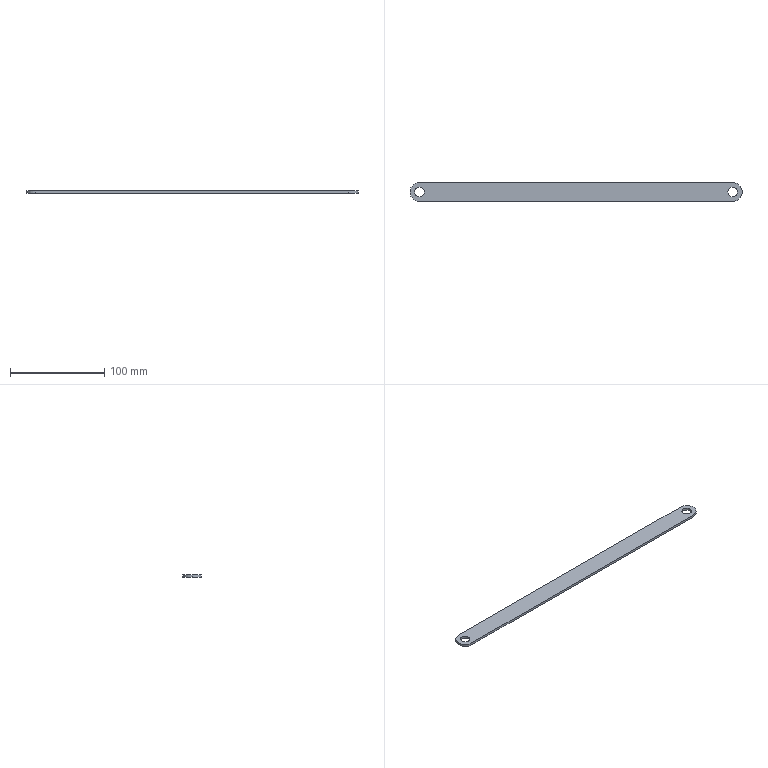Part | SolidWorks | features Extrusion 1 | 1 solid | 11 faces | box 351.77 x 20 x 2.5 mm | volume 16981 mm3 | cylinder 7 | plane 4 | commonest cylinder face diameters 10 x4 20 x3
STEP:
#1=CARTESIAN_POINT('',(160.885,0.,2.5));
#2=VERTEX_POINT('',#1);
#3=CARTESIAN_POINT('',(170.885,0.,2.5));
#4=VERTEX_POINT('',#3);
#5=CARTESIAN_POINT('',(165.885,0.,2.5));
#6=DIRECTION('',(0.,0.,1.));
#7=DIRECTION('',(1.,0.,0.));
#8=AXIS2_PLACEMENT_3D('',#5,#6,#7);
#9=CIRCLE('',#8,5.);
#10=EDGE_CURVE('',#2,#4,#9,.T.);
#11=ORIENTED_EDGE('',*,*,#10,.T.);
#12=CARTESIAN_POINT('',(170.885,0.,0.));
#13=VERTEX_POINT('',#12);
#14=CARTESIAN_POINT('',(170.885,0.,2.5));
#15=DIRECTION('',(0.,0.,-1.));
#16=VECTOR('',#15,1000.);
#17=LINE('',#14,#16);
#18=EDGE_CURVE('',#4,#13,#17,.T.);
#19=ORIENTED_EDGE('',*,*,#18,.T.);
#20=CARTESIAN_POINT('',(160.885,0.,0.));
#21=VERTEX_POINT('',#20);
#22=CARTESIAN_POINT('',(165.885,0.,0.));
#23=DIRECTION('',(0.,0.,1.));
#24=DIRECTION('',(1.,0.,0.));
#25=AXIS2_PLACEMENT_3D('',#22,#23,#24);
#26=CIRCLE('',#25,5.);
#27=EDGE_CURVE('',#21,#13,#26,.T.);
#28=ORIENTED_EDGE('',*,*,#27,.F.);
#29=CARTESIAN_POINT('',(160.885,0.,2.5));
#30=DIRECTION('',(0.,0.,-1.));
#31=VECTOR('',#30,1000.);
#32=LINE('',#29,#31);
#33=EDGE_CURVE('',#2,#21,#32,.T.);
#34=ORIENTED_EDGE('',*,*,#33,.F.);
#35=EDGE_LOOP('',(#11,#19,#28,#34));
#36=FACE_OUTER_BOUND('',#35,.T.);
#37=CARTESIAN_POINT('',(165.885,0.,2.5));
#38=DIRECTION('',(0.,0.,-1.));
#39=DIRECTION('',(-1.,0.,0.));
#40=AXIS2_PLACEMENT_3D('',#37,#38,#39);
#41=CYLINDRICAL_SURFACE('',#40,5.);
#42=ADVANCED_FACE('',(#36),#41,.F.);
#43=CARTESIAN_POINT('',(-170.885,0.,2.5));
#44=VERTEX_POINT('',#43);
#45=CARTESIAN_POINT('',(-160.885,0.,2.5));
#46=VERTEX_POINT('',#45);
#47=CARTESIAN_POINT('',(-165.885,0.,2.5));
#48=DIRECTION('',(0.,0.,1.));
#49=DIRECTION('',(1.,0.,0.));
#50=AXIS2_PLACEMENT_3D('',#47,#48,#49);
#51=CIRCLE('',#50,5.);
#52=EDGE_CURVE('',#44,#46,#51,.T.);
#53=ORIENTED_EDGE('',*,*,#52,.T.);
#54=CARTESIAN_POINT('',(-160.885,0.,0.));
#55=VERTEX_POINT('',#54);
#56=CARTESIAN_POINT('',(-160.885,0.,2.5));
#57=DIRECTION('',(0.,0.,-1.));
#58=VECTOR('',#57,1000.);
#59=LINE('',#56,#58);
#60=EDGE_CURVE('',#46,#55,#59,.T.);
#61=ORIENTED_EDGE('',*,*,#60,.T.);
#62=CARTESIAN_POINT('',(-170.885,0.,0.));
#63=VERTEX_POINT('',#62);
#64=CARTESIAN_POINT('',(-165.885,0.,0.));
#65=DIRECTION('',(0.,0.,1.));
#66=DIRECTION('',(1.,0.,0.));
#67=AXIS2_PLACEMENT_3D('',#64,#65,#66);
#68=CIRCLE('',#67,5.);
#69=EDGE_CURVE('',#63,#55,#68,.T.);
#70=ORIENTED_EDGE('',*,*,#69,.F.);
#71=CARTESIAN_POINT('',(-170.885,0.,2.5));
#72=DIRECTION('',(0.,0.,-1.));
#73=VECTOR('',#72,1000.);
#74=LINE('',#71,#73);
#75=EDGE_CURVE('',#44,#63,#74,.T.);
#76=ORIENTED_EDGE('',*,*,#75,.F.);
#77=EDGE_LOOP('',(#53,#61,#70,#76));
#78=FACE_OUTER_BOUND('',#77,.T.);
#79=CARTESIAN_POINT('',(-165.885,0.,2.5));
#80=DIRECTION('',(0.,0.,-1.));
#81=DIRECTION('',(-1.,0.,0.));
#82=AXIS2_PLACEMENT_3D('',#79,#80,#81);
#83=CYLINDRICAL_SURFACE('',#82,5.);
#84=ADVANCED_FACE('',(#78),#83,.F.);
#85=CARTESIAN_POINT('',(-175.885,0.,2.5));
#86=VERTEX_POINT('',#85);
#87=CARTESIAN_POINT('',(-165.885,-10.,2.5));
#88=VERTEX_POINT('',#87);
#89=CARTESIAN_POINT('',(-165.885,0.,2.5));
#90=DIRECTION('',(0.,0.,1.));
#91=DIRECTION('',(1.,0.,0.));
#92=AXIS2_PLACEMENT_3D('',#89,#90,#91);
#93=CIRCLE('',#92,10.);
#94=EDGE_CURVE('',#86,#88,#93,.T.);
#95=ORIENTED_EDGE('',*,*,#94,.F.);
#96=CARTESIAN_POINT('',(-175.885,0.,0.));
#97=VERTEX_POINT('',#96);
#98=CARTESIAN_POINT('',(-175.885,0.,2.5));
#99=DIRECTION('',(0.,0.,-1.));
#100=VECTOR('',#99,1000.);
#101=LINE('',#98,#100);
#102=EDGE_CURVE('',#86,#97,#101,.T.);
#103=ORIENTED_EDGE('',*,*,#102,.T.);
#104=CARTESIAN_POINT('',(-165.885,-10.,0.));
#105=VERTEX_POINT('',#104);
#106=CARTESIAN_POINT('',(-165.885,0.,0.));
#107=DIRECTION('',(0.,0.,1.));
#108=DIRECTION('',(1.,0.,0.));
#109=AXIS2_PLACEMENT_3D('',#106,#107,#108);
#110=CIRCLE('',#109,10.);
#111=EDGE_CURVE('',#97,#105,#110,.T.);
#112=ORIENTED_EDGE('',*,*,#111,.T.);
#113=CARTESIAN_POINT('',(-165.885,-10.,2.5));
#114=DIRECTION('',(0.,0.,-1.));
#115=VECTOR('',#114,1000.);
#116=LINE('',#113,#115);
#117=EDGE_CURVE('',#88,#105,#116,.T.);
#118=ORIENTED_EDGE('',*,*,#117,.F.);
#119=EDGE_LOOP('',(#95,#103,#112,#118));
#120=FACE_OUTER_BOUND('',#119,.T.);
#121=CARTESIAN_POINT('',(-165.885,0.,2.5));
#122=DIRECTION('',(0.,0.,-1.));
#123=DIRECTION('',(-1.,0.,0.));
#124=AXIS2_PLACEMENT_3D('',#121,#122,#123);
#125=CYLINDRICAL_SURFACE('',#124,10.);
#126=ADVANCED_FACE('',(#120),#125,.T.);
#127=ORIENTED_EDGE('',*,*,#52,.F.);
#128=CARTESIAN_POINT('',(-165.885,0.,2.5));
#129=DIRECTION('',(0.,0.,1.));
#130=DIRECTION('',(1.,0.,0.));
#131=AXIS2_PLACEMENT_3D('',#128,#129,#130);
#132=CIRCLE('',#131,5.);
#133=EDGE_CURVE('',#46,#44,#132,.T.);
#134=ORIENTED_EDGE('',*,*,#133,.F.);
#135=EDGE_LOOP('',(#127,#134));
#136=FACE_BOUND('',#135,.T.);
#137=CARTESIAN_POINT('',(-165.885,10.,2.5));
#138=VERTEX_POINT('',#137);
#139=CARTESIAN_POINT('',(-165.885,0.,2.5));
#140=DIRECTION('',(0.,0.,1.));
#141=DIRECTION('',(1.,0.,0.));
#142=AXIS2_PLACEMENT_3D('',#139,#140,#141);
#143=CIRCLE('',#142,10.);
#144=EDGE_CURVE('',#138,#86,#143,.T.);
#145=ORIENTED_EDGE('',*,*,#144,.T.);
#146=ORIENTED_EDGE('',*,*,#94,.T.);
#147=CARTESIAN_POINT('',(165.885,-10.,2.5));
#148=VERTEX_POINT('',#147);
#149=CARTESIAN_POINT('',(-165.885,-10.,2.5));
#150=DIRECTION('',(1.,0.,0.));
#151=VECTOR('',#150,1000.);
#152=LINE('',#149,#151);
#153=EDGE_CURVE('',#88,#148,#152,.T.);
#154=ORIENTED_EDGE('',*,*,#153,.T.);
#155=CARTESIAN_POINT('',(165.885,10.,2.5));
#156=VERTEX_POINT('',#155);
#157=CARTESIAN_POINT('',(165.885,0.,2.5));
#158=DIRECTION('',(0.,0.,1.));
#159=DIRECTION('',(1.,0.,0.));
#160=AXIS2_PLACEMENT_3D('',#157,#158,#159);
#161=CIRCLE('',#160,10.);
#162=EDGE_CURVE('',#148,#156,#161,.T.);
#163=ORIENTED_EDGE('',*,*,#162,.T.);
#164=CARTESIAN_POINT('',(-165.885,10.,2.5));
#165=DIRECTION('',(-1.,0.,0.));
#166=VECTOR('',#165,1000.);
#167=LINE('',#164,#166);
#168=EDGE_CURVE('',#156,#138,#167,.T.);
#169=ORIENTED_EDGE('',*,*,#168,.T.);
#170=EDGE_LOOP('',(#145,#146,#154,#163,#169));
#171=FACE_OUTER_BOUND('',#170,.T.);
#172=ORIENTED_EDGE('',*,*,#10,.F.);
#173=CARTESIAN_POINT('',(165.885,0.,2.5));
#174=DIRECTION('',(0.,0.,1.));
#175=DIRECTION('',(1.,0.,0.));
#176=AXIS2_PLACEMENT_3D('',#173,#174,#175);
#177=CIRCLE('',#176,5.);
#178=EDGE_CURVE('',#4,#2,#177,.T.);
#179=ORIENTED_EDGE('',*,*,#178,.F.);
#180=EDGE_LOOP('',(#172,#179));
#181=FACE_BOUND('',#180,.T.);
#182=CARTESIAN_POINT('',(-165.885,0.,2.5));
#183=DIRECTION('',(0.,0.,1.));
#184=DIRECTION('',(1.,0.,0.));
#185=AXIS2_PLACEMENT_3D('',#182,#183,#184);
#186=PLANE('',#185);
#187=ADVANCED_FACE('',(#136,#171,#181),#186,.T.);
#188=CARTESIAN_POINT('',(-165.885,10.,0.));
#189=VERTEX_POINT('',#188);
#190=CARTESIAN_POINT('',(-165.885,0.,0.));
#191=DIRECTION('',(0.,0.,1.));
#192=DIRECTION('',(1.,0.,0.));
#193=AXIS2_PLACEMENT_3D('',#190,#191,#192);
#194=CIRCLE('',#193,10.);
#195=EDGE_CURVE('',#189,#97,#194,.T.);
#196=ORIENTED_EDGE('',*,*,#195,.F.);
#197=CARTESIAN_POINT('',(165.885,10.,0.));
#198=VERTEX_POINT('',#197);
#199=CARTESIAN_POINT('',(-165.885,10.,0.));
#200=DIRECTION('',(-1.,0.,0.));
#201=VECTOR('',#200,1000.);
#202=LINE('',#199,#201);
#203=EDGE_CURVE('',#198,#189,#202,.T.);
#204=ORIENTED_EDGE('',*,*,#203,.F.);
#205=CARTESIAN_POINT('',(165.885,-10.,0.));
#206=VERTEX_POINT('',#205);
#207=CARTESIAN_POINT('',(165.885,0.,0.));
#208=DIRECTION('',(0.,0.,1.));
#209=DIRECTION('',(1.,0.,0.));
#210=AXIS2_PLACEMENT_3D('',#207,#208,#209);
#211=CIRCLE('',#210,10.);
#212=EDGE_CURVE('',#206,#198,#211,.T.);
#213=ORIENTED_EDGE('',*,*,#212,.F.);
#214=CARTESIAN_POINT('',(-165.885,-10.,0.));
#215=DIRECTION('',(1.,0.,0.));
#216=VECTOR('',#215,1000.);
#217=LINE('',#214,#216);
#218=EDGE_CURVE('',#105,#206,#217,.T.);
#219=ORIENTED_EDGE('',*,*,#218,.F.);
#220=ORIENTED_EDGE('',*,*,#111,.F.);
#221=EDGE_LOOP('',(#196,#204,#213,#219,#220));
#222=FACE_OUTER_BOUND('',#221,.T.);
#223=ORIENTED_EDGE('',*,*,#69,.T.);
#224=CARTESIAN_POINT('',(-165.885,0.,0.));
#225=DIRECTION('',(0.,0.,1.));
#226=DIRECTION('',(1.,0.,0.));
#227=AXIS2_PLACEMENT_3D('',#224,#225,#226);
#228=CIRCLE('',#227,5.);
#229=EDGE_CURVE('',#55,#63,#228,.T.);
#230=ORIENTED_EDGE('',*,*,#229,.T.);
#231=EDGE_LOOP('',(#223,#230));
#232=FACE_BOUND('',#231,.T.);
#233=ORIENTED_EDGE('',*,*,#27,.T.);
#234=CARTESIAN_POINT('',(165.885,0.,0.));
#235=DIRECTION('',(0.,0.,1.));
#236=DIRECTION('',(1.,0.,0.));
#237=AXIS2_PLACEMENT_3D('',#234,#235,#236);
#238=CIRCLE('',#237,5.);
#239=EDGE_CURVE('',#13,#21,#238,.T.);
#240=ORIENTED_EDGE('',*,*,#239,.T.);
#241=EDGE_LOOP('',(#233,#240));
#242=FACE_BOUND('',#241,.T.);
#243=CARTESIAN_POINT('',(-165.885,0.,0.));
#244=DIRECTION('',(0.,0.,1.));
#245=DIRECTION('',(1.,0.,0.));
#246=AXIS2_PLACEMENT_3D('',#243,#244,#245);
#247=PLANE('',#246);
#248=ADVANCED_FACE('',(#222,#232,#242),#247,.F.);
#249=ORIENTED_EDGE('',*,*,#102,.F.);
#250=ORIENTED_EDGE('',*,*,#144,.F.);
#251=CARTESIAN_POINT('',(-165.885,10.,2.5));
#252=DIRECTION('',(0.,0.,-1.));
#253=VECTOR('',#252,1000.);
#254=LINE('',#251,#253);
#255=EDGE_CURVE('',#138,#189,#254,.T.);
#256=ORIENTED_EDGE('',*,*,#255,.T.);
#257=ORIENTED_EDGE('',*,*,#195,.T.);
#258=EDGE_LOOP('',(#249,#250,#256,#257));
#259=FACE_OUTER_BOUND('',#258,.T.);
#260=CARTESIAN_POINT('',(-165.885,0.,2.5));
#261=DIRECTION('',(0.,0.,-1.));
#262=DIRECTION('',(-1.,0.,0.));
#263=AXIS2_PLACEMENT_3D('',#260,#261,#262);
#264=CYLINDRICAL_SURFACE('',#263,10.);
#265=ADVANCED_FACE('',(#259),#264,.T.);
#266=ORIENTED_EDGE('',*,*,#218,.T.);
#267=CARTESIAN_POINT('',(165.885,-10.,2.5));
#268=DIRECTION('',(0.,0.,-1.));
#269=VECTOR('',#268,1000.);
#270=LINE('',#267,#269);
#271=EDGE_CURVE('',#148,#206,#270,.T.);
#272=ORIENTED_EDGE('',*,*,#271,.F.);
#273=ORIENTED_EDGE('',*,*,#153,.F.);
#274=ORIENTED_EDGE('',*,*,#117,.T.);
#275=EDGE_LOOP('',(#266,#272,#273,#274));
#276=FACE_OUTER_BOUND('',#275,.T.);
#277=CARTESIAN_POINT('',(-165.885,-10.,2.5));
#278=DIRECTION('',(0.,1.,0.));
#279=DIRECTION('',(0.,0.,1.));
#280=AXIS2_PLACEMENT_3D('',#277,#278,#279);
#281=PLANE('',#280);
#282=ADVANCED_FACE('',(#276),#281,.F.);
#283=ORIENTED_EDGE('',*,*,#212,.T.);
#284=CARTESIAN_POINT('',(165.885,10.,2.5));
#285=DIRECTION('',(0.,0.,-1.));
#286=VECTOR('',#285,1000.);
#287=LINE('',#284,#286);
#288=EDGE_CURVE('',#156,#198,#287,.T.);
#289=ORIENTED_EDGE('',*,*,#288,.F.);
#290=ORIENTED_EDGE('',*,*,#162,.F.);
#291=ORIENTED_EDGE('',*,*,#271,.T.);
#292=EDGE_LOOP('',(#283,#289,#290,#291));
#293=FACE_OUTER_BOUND('',#292,.T.);
#294=CARTESIAN_POINT('',(165.885,0.,2.5));
#295=DIRECTION('',(0.,0.,-1.));
#296=DIRECTION('',(-1.,0.,0.));
#297=AXIS2_PLACEMENT_3D('',#294,#295,#296);
#298=CYLINDRICAL_SURFACE('',#297,10.);
#299=ADVANCED_FACE('',(#293),#298,.T.);
#300=ORIENTED_EDGE('',*,*,#203,.T.);
#301=ORIENTED_EDGE('',*,*,#255,.F.);
#302=ORIENTED_EDGE('',*,*,#168,.F.);
#303=ORIENTED_EDGE('',*,*,#288,.T.);
#304=EDGE_LOOP('',(#300,#301,#302,#303));
#305=FACE_OUTER_BOUND('',#304,.T.);
#306=CARTESIAN_POINT('',(-165.885,10.,2.5));
#307=DIRECTION('',(0.,-1.,0.));
#308=DIRECTION('',(0.,0.,-1.));
#309=AXIS2_PLACEMENT_3D('',#306,#307,#308);
#310=PLANE('',#309);
#311=ADVANCED_FACE('',(#305),#310,.F.);
#312=ORIENTED_EDGE('',*,*,#60,.F.);
#313=ORIENTED_EDGE('',*,*,#133,.T.);
#314=ORIENTED_EDGE('',*,*,#75,.T.);
#315=ORIENTED_EDGE('',*,*,#229,.F.);
#316=EDGE_LOOP('',(#312,#313,#314,#315));
#317=FACE_OUTER_BOUND('',#316,.T.);
#318=CARTESIAN_POINT('',(-165.885,0.,2.5));
#319=DIRECTION('',(0.,0.,-1.));
#320=DIRECTION('',(-1.,0.,0.));
#321=AXIS2_PLACEMENT_3D('',#318,#319,#320);
#322=CYLINDRICAL_SURFACE('',#321,5.);
#323=ADVANCED_FACE('',(#317),#322,.F.);
#324=ORIENTED_EDGE('',*,*,#18,.F.);
#325=ORIENTED_EDGE('',*,*,#178,.T.);
#326=ORIENTED_EDGE('',*,*,#33,.T.);
#327=ORIENTED_EDGE('',*,*,#239,.F.);
#328=EDGE_LOOP('',(#324,#325,#326,#327));
#329=FACE_OUTER_BOUND('',#328,.T.);
#330=CARTESIAN_POINT('',(165.885,0.,2.5));
#331=DIRECTION('',(0.,0.,-1.));
#332=DIRECTION('',(-1.,0.,0.));
#333=AXIS2_PLACEMENT_3D('',#330,#331,#332);
#334=CYLINDRICAL_SURFACE('',#333,5.);
#335=ADVANCED_FACE('',(#329),#334,.F.);
#336=CLOSED_SHELL('',(#42,#84,#126,#187,#248,#265,#282,#299,#311,#323,#335));
#337=MANIFOLD_SOLID_BREP('',#336);
#338=CARTESIAN_POINT('',(0.,0.,0.));
#339=DIRECTION('',(0.,0.,1.));
#340=DIRECTION('',(1.,0.,0.));
#341=AXIS2_PLACEMENT_3D('',#338,#339,#340);
#342=(LENGTH_UNIT()NAMED_UNIT(*)SI_UNIT(.MILLI.,.METRE.));
#343=UNCERTAINTY_MEASURE_WITH_UNIT(LENGTH_MEASURE(0.00001),#342,'','');
#344=(NAMED_UNIT(*)PLANE_ANGLE_UNIT()SI_UNIT($,.RADIAN.));
#345=(NAMED_UNIT(*)SI_UNIT($,.STERADIAN.)SOLID_ANGLE_UNIT());
#346=(GEOMETRIC_REPRESENTATION_CONTEXT(3)GLOBAL_UNCERTAINTY_ASSIGNED_CONTEXT((#343))GLOBAL_UNIT_ASSIGNED_CONTEXT((#342,#344,#345))REPRESENTATION_CONTEXT('',''));
#347=ADVANCED_BREP_SHAPE_REPRESENTATION('',(#337,#341),#346);